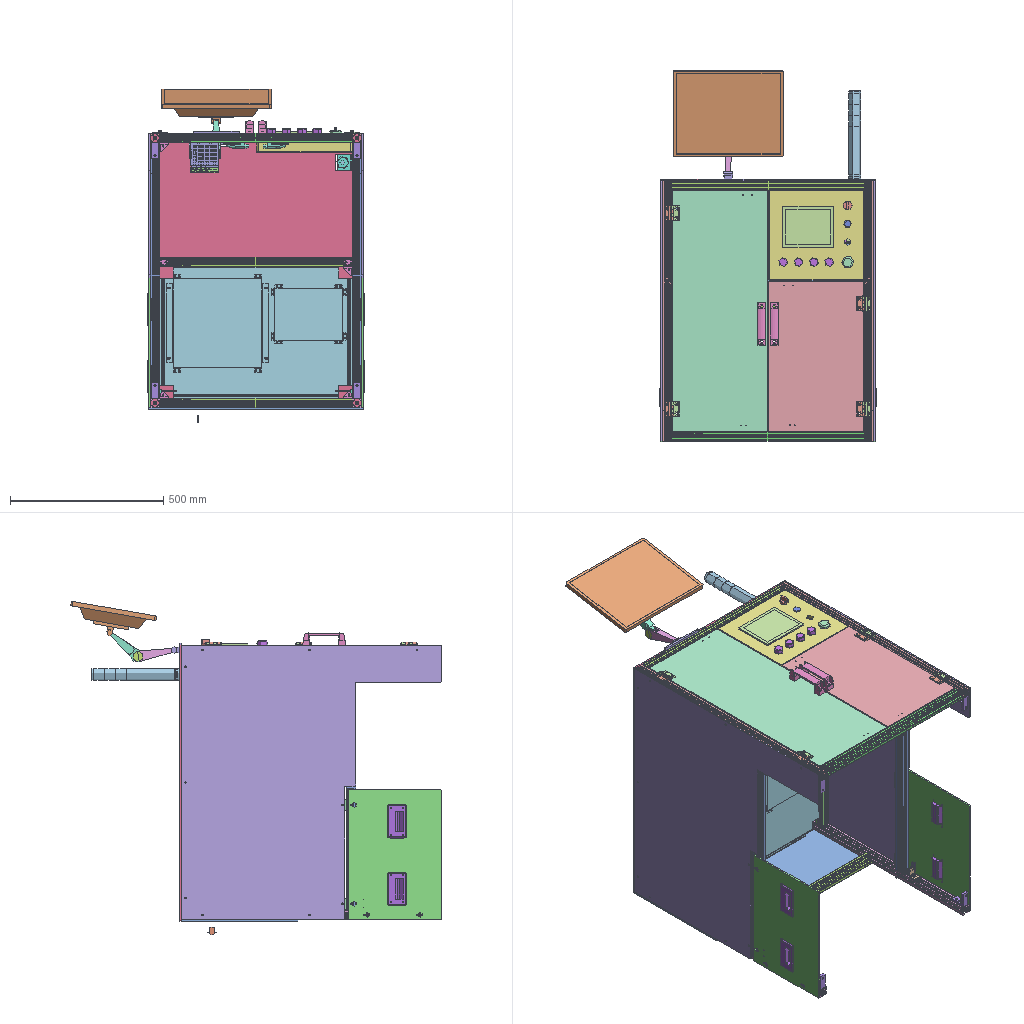Assembly | STEP file | 62 different items | 138 placed | box 710 x 1211 x 1090 mm
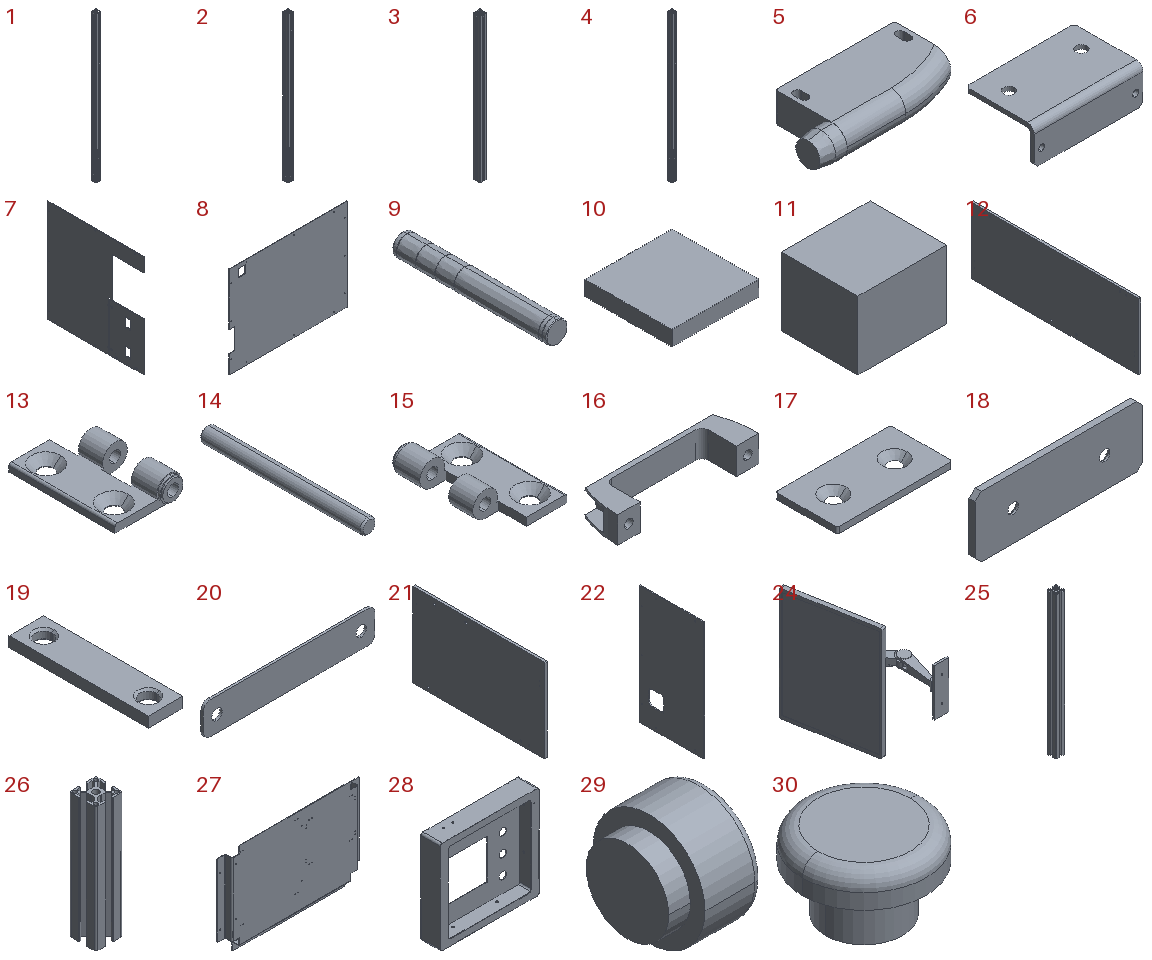Parts list (item | name | quantity | parent item | size | volume):
1 | 227H056139_Default | x2 | in 20 | 30 x 30 x 850 mm | 322963 mm3
2 | SQ-8-3030W-835_Default | x4 | in 20 | 30 x 30 x 835 mm | 317751 mm3
3 | SQ-8-3030W-630_Default | x4 | in 20 | 30 x 30 x 630 mm | 238380 mm3
4 | SQ-8-3030W-850_Default | x2 | in 20 | 30 x 30 x 850 mm | 323559 mm3
5 | AZC11013Y_Default | x2 | in 20 | 72.7 x 40.3 x 15 mm | 31534 mm3
6 | 227H056122 Sensor BKT_Default | x1 | in 20 | 60 x 38 x 20 mm | 7342 mm3
7 | 227H056116 Side Cover _Default | x2 | in 20 | 5 x 849 x 893 mm | 3234817 mm3
8 | 227H056117 Top Cover_Default | x1 | in 20 | 900 x 5 x 700 mm | 3097744 mm3
9 | SceondRR_Default | x1 | in 20 | 40 x 289 x 40 mm | 362543 mm3
10 | SceondUPS_Default | x1 | in 20 | 290 x 290 x 50 mm | 4205000 mm3
11 | SceondREWTRT_Default | x1 | in 20 | 220 x 190 x 170 mm | 7106000 mm3
12 | 227H056118 DOOR L_Default | x1 | in DOOR L_Default | 10 x 786 x 311 mm | 2441721 mm3
13 | SecondRearHHPMGS6p1_Default | x4 | in HHPMGS6_Default | 29.5 x 48.7 x 11 mm | 4355 mm3
14 | SecondRearHHPMGS6pin_Default | x4 | in HHPMGS6_Default | 5 x 54 x 5 mm | 1057 mm3
15 | SecondRearHHPMGS6p2_Default | x4 | in HHPMGS6_Default | 29.5 x 48.7 x 11 mm | 4355 mm3
16 | SecondRearUPCN26-B-41_b_Default | x2 | in DOOR L_Default, DOOR R_Default | 139 x 41 x 26 mm | 37829 mm3
17 | SceondC-100-B-2Receiving Plate_Default | x2 | in DOOR L_Default, DOOR R_Default | 30 x 16 x 1.6 mm | 705.168 mm3
18 | Part1.SLDPRTrtt_Default | x2 | in DOOR L_Default, DOOR R_Default | 55 x 2 x 20 mm | 2119 mm3
19 | hhpnt6_2_2_03 | x4 | in DOOR L_Default, DOOR R_Default | 10 x 40 x 3 mm | 1076 mm3
20 | upcnat117_2_03 | x2 | in DOOR L_Default, DOOR R_Default | 139 x 2 x 26 mm | 6946 mm3
21 | 227H056119 DOOR R_Default | x1 | in DOOR R_Default | 10 x 491 x 311 mm | 1524271 mm3
22 | 227H056124 Rear Cover SLDPRT_Default | x1 | in 20 | 5 x 380 x 700 mm | 1290724 mm3
23 | 0-ARK-3500_Default | x1 | in 20 | - | -
24 | TV | x1 | in 20 | 197.95 x 360.761 x 359.449 mm | 3578288 mm3
25 | SQ-8-3030W-460_Default | x2 | in 20 | 30 x 30 x 460 mm | 172560 mm3
26 | SQ-8-3030W-160_Default | x2 | in 20 | 30 x 30 x 140 mm | 48663 mm3
27 | 227H056121 BKT_Default | x1 | in 20 | 685.4 x 35.3 x 457.7 mm | 768690 mm3
28 | 227H056120A Front Panel | x1 | in Front Panel | 313 x 61.6 x 295 mm | 263384 mm3
29 | 7-4-Part3-619-724 | x4 | in Front Panel | 21.06 x 29.813 x 29.813 mm | 12789 mm3
30 | 7-4-Emergency Stop Button1-619-724_Default | x1 | in Front Panel | 40 x 40 x 25 mm | 19293 mm3
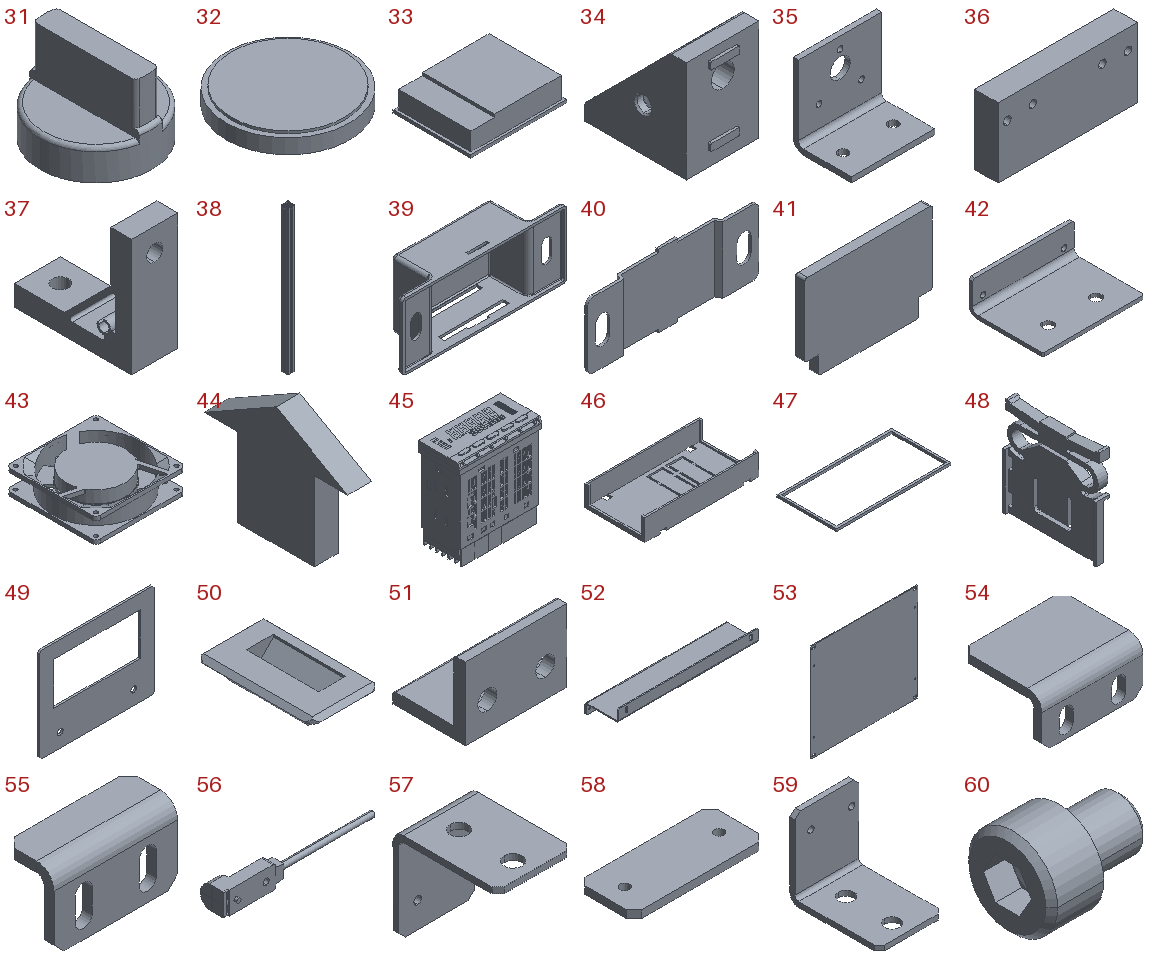31 | 7-4-Switch1-619-724_Default | x1 | in Front Panel | 29 x 29 x 21 mm | 7372 mm3
32 | 7-4-Button1-619-724_Default | x1 | in Front Panel | 25 x 25 x 3.5 mm | 1680 mm3
33 | Display-724_Default | x1 | in Front Panel | 165 x 134 x 41 mm | 776017 mm3
34 | - | x19 | in 20 | 20 x 28.7 x 28.7 mm | 5707 mm3
35 | 203H124123 Signal Tower BKT_Default | x1 | in 20 | 50 x 35 x 48 mm | 11822 mm3
36 | 227H056123 Block_Default | x1 | in 20 | 60 x 10 x 30 mm | 17658 mm3
37 | hblts6_2_03 | x4 | in 20 | 20 x 51 x 51 mm | 16227 mm3
38 | SQ-8-3030W-630 Bottom_Default | x1 | in 20 | 30 x 30 x 630 mm | 237831 mm3
39 | SceondC-100-B-2Case_Default | x2 | in SceondC-100-B-2, C-100-B-2 | 56.5 x 15.3 x 23 mm | 2154 mm3
40 | SceondC-100-B-2Base Plate_Default | x2 | in SceondC-100-B-2, C-100-B-2 | 54.5 x 2.5 x 23 mm | 897.584 mm3
41 | SceondC-100-BYoke_Default | x2 | in SceondC-100-BYoke_Male_Default | 28 x 2 x 20 mm | 1071 mm3
42 | 227H056396 BKT_Default | x2 | in 20 | 56.5 x 41.063 x 18 mm | 6109 mm3
43 | 1_2_1-- | x1 | in E0141_Default | 92 x 92 x 25 mm | 97841 mm3
44 | 2_2_1-- | x1 | in E0141_Default | 5 x 30 x 25 mm | 1957 mm3
45 | K3HB_V_BASE | x1 | in K3HB_V | 96 x 48 x 108.3 mm | 416393 mm3
46 | K3HB_V_COVER. | x1 | in K3HB_V | 91 x 47.87 x 17 mm | 10803 mm3
47 | K3HB_V_PACKING | x1 | in K3HB_V | 95 x 48.8 x 2 mm | 1118 mm3
48 | K3HB_V_ADAPTER | x2 | in K3HB_V | 6.7 x 47.4 x 49.3 mm | 5859 mm3
49 | 227H0563998 BKT_Default | x1 | in K3HB_V | 122 x 2 x 100 mm | 15991 mm3
50 | uwuan109_5_n_2_14a | x4 | in 20 | 64 x 109.5 x 19.5 mm | 44747 mm3
51 | hcba6_2_14a_Default | x4 | in 20 | 35 x 25 x 25 mm | 6095 mm3
52 | 227H056377 Guide BKT_Default | x2 | in 20 | 260 x 62 x 40 mm | 50446 mm3
53 | 227H056376 BKT_Default | x1 | in 20 | 285 x 2 x 260 mm | 147758 mm3
54 | 227H056379 BKT_Default | x8 | in 20 | 25 x 20 x 12 mm | 1357 mm3
55 | 227H056378 BKT_Default | x4 | in 20 | 25 x 10 x 15 mm | 978.865 mm3
56 | gx-h12a | x2 | in 20 | 81.8 x 14.5 x 12 mm | 2908 mm3
57 | 227H056375 Sensor BKT_Default | x1 | in 20 | 25 x 35 x 31 mm | 2998 mm3
58 | 227H056374 Sensor Dog_Default | x2 | in 20 | 35 x 15 x 2 mm | 1014 mm3
59 | 227H056373 Sensor BKT_Default | x1 | in 20 | 25 x 35 x 31 mm | 2998 mm3
60 | CB5-6_Default | x1 | in CB5-6_SW5_W5_Default | 11 x 8.5 x 8.5 mm | 358.786 mm3
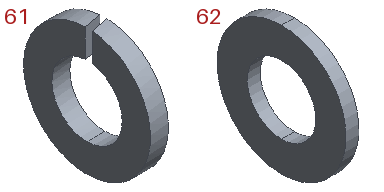61 | SW5_Default | x1 | in CB5-6_SW5_W5_Default | 1.3 x 9.2 x 9.198 mm | 58.481 mm3
62 | W5_Default | x1 | in CB5-6_SW5_W5_Default | 1 x 10 x 10 mm | 56.478 mm3
Placements (level | parent | child | x y z in mm | rotation matrix by rows):
1 | 20 | 227H056139_Default | -330.0 175.4 435.0 | -1 0 0 0 0 -1 0 -1 0
1 | 20 | SQ-8-3030W-835_Default | -330.0 835.0 244.6 | 1 0 0 0 1 0 0 0 1
1 | 20 | SQ-8-3030W-835_Default | 330.0 835.0 244.6 | 1 0 0 0 1 0 0 0 1
1 | 20 | SQ-8-3030W-630_Default | -139.6 835.0 -430.0 | 0 0 -1 -1 0 0 0 1 -0
1 | 20 | SQ-8-3030W-630_Default | -139.6 835.0 435.0 | 0 0 -1 -1 0 0 0 1 -0
1 | 20 | 227H056139_Default | 330.0 175.4 435.0 | 1 0 0 0 0 -1 0 1 0
1 | 20 | SQ-8-3030W-850_Default | -330.0 674.6 -430.0 | 0 1 0 0 0 1 1 0 0
1 | 20 | SQ-8-3030W-850_Default | 330.0 674.6 -430.0 | 0 1 0 0 0 1 1 0 0
1 | 20 | AZC11013Y_Default | -37 796.0 401.389 | -1 0 0 0 0 1 0 1 -0
1 | 20 | 227H056122 Sensor BKT_Default | -66.999 811.0 414.7 | -1 0 0 0 1 0 0 0 -1
1 | 20 | AZC11013Y_Default | 37 515.0 400.411 | 1 0 0 0 0 -1 0 1 -0
1 | 20 | 227H056116 Side Cover _Default | -350.0 424.5 2.5 | 1 0 0 0 1 0 0 0 1
1 | 20 | 227H056116 Side Cover _Default | 345.0 424.5 2.5 | 1 0 0 0 1 0 0 0 1
1 | 20 | 227H056117 Top Cover_Default | -0.0 850.0 -0.0 | 0 0 1 0 1 0 -1 0 0
1 | 20 | SceondRR_Default | 283.5 855.0 355.0 | -0.9502 0 0.3116 0 1 0 -0.3116 0 -0.9502
1 | 20 | SceondUPS_Default | -270.7 699.3 -25.0 | 1 0 0 0 0 1 0 -1 0
1 | 20 | SceondREWTRT_Default | 172.0 649.3 -140.0 | -1 0 0 0 1 0 0 0 -1
1 | 20 | DOOR L_Default | -157.5 425.0 440.0 | 0 0 -1 0 1 0 1 0 -0
2 | DOOR L_Default | 227H056118 DOOR L_Default | -0.0 -0.0 -0.0 | 1 0 0 0 1 0 0 0 1
2 | DOOR L_Default | HHPMGS6_Default | 15.5 319.5 156.5 | 0 0 1 0 1 0 -1 0 -0
3 | HHPMGS6_Default | SecondRearHHPMGS6p1_Default | 0.0 0.0 -0.0 | 1 0 0 0 1 0 0 0 1
3 | HHPMGS6_Default | SecondRearHHPMGS6pin_Default | 0.0 0.0 -0.0 | 1 0 0 0 1 0 0 0 1
3 | HHPMGS6_Default | SecondRearHHPMGS6p2_Default | 0.0 0.0 -0.0 | 1 0 0 0 1 0 0 0 1
2 | DOOR L_Default | SecondRearUPCN26-B-41_b_Default | 10.0 16.3 -137.5 | 0 1 0 -1 0 0 0 0 1
2 | DOOR L_Default | HHPMGS6_Default | 15.5 -319.5 156.5 | 0 0 1 0 1 0 -1 0 -0
3 | HHPMGS6_Default | SecondRearHHPMGS6p1_Default | 0.0 0.0 -0.0 | 1 0 0 0 1 0 0 0 1
3 | HHPMGS6_Default | SecondRearHHPMGS6pin_Default | 0.0 0.0 -0.0 | 1 0 0 0 1 0 0 0 1
3 | HHPMGS6_Default | SecondRearHHPMGS6p2_Default | 0.0 0.0 -0.0 | 1 0 0 0 1 0 0 0 1
2 | DOOR L_Default | SceondC-100-B-2Receiving Plate_Default | -1.6 -381.7 -78.2 | 0 0 -1 0 1 0 1 0 -0
2 | DOOR L_Default | Part1.SLDPRTrtt_Default | -0.0 378.0 -90.5 | 0 -1 0 0 0 -1 1 0 0
2 | DOOR L_Default | hhpnt6_2_2_03 | 0.0 319.5 140.5 | 0 0 -1 0 1 0 1 0 0
2 | DOOR L_Default | hhpnt6_2_2_03 | -0.0 -319.5 140.5 | 0 0 -1 0 1 0 1 0 0
2 | DOOR L_Default | upcnat117_2_03 | 0.0 -42.2 -137.5 | 0 -1 0 1 0 0 0 0 1
1 | 20 | DOOR R_Default | 157.5 277.5 440.0 | 0 0 -1 0 1 0 1 0 -0
2 | DOOR R_Default | 227H056119 DOOR R_Default | -0.0 -0.0 -0.0 | 1 0 0 0 1 0 0 0 1
2 | DOOR R_Default | SecondRearUPCN26-B-41_b_Default | 10.0 46.8 137.5 | 0 1 0 1 0 0 0 0 -1
2 | DOOR R_Default | SceondC-100-B-2Receiving Plate_Default | -1.6 -233.7 78.2 | 0 0 -1 0 1 0 1 0 -0
2 | DOOR R_Default | HHPMGS6_Default | 15.5 -172.0 -156.5 | 0 0 1 0 1 0 -1 0 -0
3 | HHPMGS6_Default | SecondRearHHPMGS6p1_Default | 0.0 0.0 -0.0 | 1 0 0 0 1 0 0 0 1
3 | HHPMGS6_Default | SecondRearHHPMGS6pin_Default | 0.0 0.0 -0.0 | 1 0 0 0 1 0 0 0 1
3 | HHPMGS6_Default | SecondRearHHPMGS6p2_Default | 0.0 0.0 -0.0 | 1 0 0 0 1 0 0 0 1
2 | DOOR R_Default | HHPMGS6_Default | 15.5 172.0 -156.5 | 0 0 1 0 1 0 -1 0 -0
3 | HHPMGS6_Default | SecondRearHHPMGS6p1_Default | 0.0 0.0 -0.0 | 1 0 0 0 1 0 0 0 1
3 | HHPMGS6_Default | SecondRearHHPMGS6pin_Default | 0.0 0.0 -0.0 | 1 0 0 0 1 0 0 0 1
3 | HHPMGS6_Default | SecondRearHHPMGS6p2_Default | 0.0 0.0 -0.0 | 1 0 0 0 1 0 0 0 1
2 | DOOR R_Default | Part1.SLDPRTrtt_Default | 0.0 230.5 90.5 | 0 -1 0 0 0 -1 1 0 -0
2 | DOOR R_Default | hhpnt6_2_2_03 | -0.0 172.0 -140.5 | 0 0 -1 0 -1 0 -1 0 0
2 | DOOR R_Default | hhpnt6_2_2_03 | 0.0 -172.0 -140.5 | 0 0 -1 0 -1 0 -1 0 0
2 | DOOR R_Default | upcnat117_2_03 | -2.0 105.3 137.5 | 0 1 0 -1 0 0 0 0 1
1 | 20 | 227H056124 Rear Cover SLDPRT_Default | -0.0 659.0 -445.0 | 0 0 1 0 1 0 -1 0 0
1 | 20 | 0-ARK-3500_Default | -125 776.3 -57.0 | 1 0 0 0 1 0 0 0 1
1 | 20 | TV | -130.0 991.0 414.162 | 0 0 1 0 1 0 -1 0 0
1 | 20 | SQ-8-3030W-630_Default | -139.6 835.0 30.0 | 0 0 -1 -1 0 0 0 1 -0
1 | 20 | SQ-8-3030W-460_Default | -330.0 665.0 -130.4 | 1 0 0 0 1 0 0 0 1
1 | 20 | SQ-8-3030W-460_Default | 330.0 665.0 -130.4 | 1 0 0 0 1 0 0 0 1
1 | 20 | SQ-8-3030W-160_Default | -330.0 855.4 30.0 | 1 0 0 0 0 -1 0 1 -0
1 | 20 | SQ-8-3030W-160_Default | 330.0 855.4 30.0 | 1 0 0 0 0 -1 0 1 -0
1 | 20 | 227H056121 BKT_Default | -0.0 649.3 -197.3 | 1 0 0 0 1 0 0 0 1
1 | 20 | SQ-8-3030W-630_Default | -139.6 431.238 -430.0 | 0 0 -1 -1 0 0 0 1 -0
1 | 20 | Front Panel | 353.404 -309.683 99.086 | 0.9984 -0.05571 0.009823 0.05657 0.9832 -0.1734 0 0.1736 0.9848
2 | Front Panel | 227H056120A Front Panel | -158.206 1026.246 175.373 | 0.9984 0 -0.05657 -0.05571 0.1736 -0.9832 0.009823 0.9848 0.1734
2 | Front Panel | 7-4-Part3-619-724 | -254.243 966.693 180.016 | 0 -0.1736 -0.9848 0.1736 0.9698 -0.171 0.9848 -0.171 0.03015
2 | Front Panel | 7-4-Part3-619-724 | -204.323 963.907 180.507 | 0 -0.1736 -0.9848 0.1736 0.9698 -0.171 0.9848 -0.171 0.03015
2 | Front Panel | 7-4-Part3-619-724 | -154.404 961.122 180.998 | 0 -0.1736 -0.9848 0.1736 0.9698 -0.171 0.9848 -0.171 0.03015
2 | Front Panel | 7-4-Part3-619-724 | -104.484 958.336 181.489 | 0 -0.1736 -0.9848 0.1736 0.9698 -0.171 0.9848 -0.171 0.03015
2 | Front Panel | 7-4-Emergency Stop Button1-619-724_Default | -42.67 947.063 199.489 | 1 0 0 0 0.9848 0.1736 0 -0.1736 0.9848
2 | Front Panel | 7-4-Switch1-619-724_Default | -32.204 1130.871 178.249 | 1 0 0 0 0.9848 0.1736 0 -0.1736 0.9848
2 | Front Panel | 7-4-Button1-619-724_Default | -35.598 1068.752 170.924 | 1 0 0 0 0.9848 0.1736 0 -0.1736 0.9848
2 | Front Panel | Display-724_Default | -177.335 1078.541 171.229 | 0.9984 -0.05657 0 -0.05571 -0.9832 -0.1736 0.009823 0.1734 -0.9848
1 | 20 | subassembly 2 | -330.0 820.0 -415.0 | 1 0 0 0 0 -1 0 1 0
1 | 20 | subassembly 2 | -330.0 680.0 -415.0 | -1 0 0 0 0 1 0 1 -0
1 | 20 | subassembly 2 | -330.0 680.0 15.0 | -1 0 0 0 1 0 0 0 -1
1 | 20 | subassembly 2 | -330.0 820.0 15.0 | -1 0 0 0 0 -1 0 -1 -0
1 | 20 | subassembly 2 | 330.0 820.0 420.0 | -1 0 0 0 0 -1 0 -1 0
1 | 20 | subassembly 2 | 330.0 820.0 45.0 | -1 0 0 0 -1 0 0 0 1
1 | 20 | subassembly 2 | 315.0 680.0 30.0 | 0 0 -1 0 1 0 1 0 0
1 | 20 | subassembly 2 | -315.0 680.0 30.0 | 0 0 1 0 1 0 -1 0 0
1 | 20 | subassembly 2 | 315.0 665.0 15.0 | 0 0 -1 1 0 0 0 -1 -0
1 | 20 | subassembly 2 | 315.0 820.0 30.0 | 0 -1 0 0 0 -1 1 0 -0
1 | 20 | subassembly 2 | -315.0 820.0 30.0 | 0 1 0 0 0 -1 -1 0 -0
1 | 20 | subassembly 2 | -330.0 820.0 45.0 | -1 0 0 0 -1 0 0 0 1
1 | 20 | subassembly 2 | -330.0 820.0 420.0 | -1 0 0 0 0 -1 0 -1 0
1 | 20 | subassembly 2 | 315.0 820.0 -430.0 | 0 -1 0 0 0 -1 1 0 -0
1 | 20 | subassembly 2 | -315.0 820.0 -430.0 | 0 1 0 0 0 -1 -1 0 -0
1 | 20 | subassembly 2 | -315.0 835.0 420.0 | 0 1 0 1 0 0 0 0 -1
1 | 20 | subassembly 2 | 315.0 835.0 420.0 | 0 0 -1 1 0 0 0 -1 -0
1 | 20 | subassembly 2 | 315.0 835.0 -415.0 | 0 0 -1 -1 0 0 0 1 -0
1 | 20 | subassembly 2 | -315.0 835.0 -415.0 | 0 1 0 -1 0 0 0 0 1
1 | 20 | 203H124123 Signal Tower BKT_Default | 315.0 820.0 355.0 | 0 0 -1 0 1 0 1 0 -0
1 | 20 | 227H056123 Block_Default | 67.0 515.0 421.3 | 1 0 0 0 1 0 0 0 1
1 | 20 | hblts6_2_03 | -330.0 0.0 420.0 | 1 0 0 0 0 1 0 -1 -0
1 | 20 | hblts6_2_03 | 330.0 0.0 420.0 | 1 0 0 0 0 1 0 -1 -0
1 | 20 | hblts6_2_03 | 330.0 0.0 -415.0 | -1 0 0 0 0 1 0 1 -0
1 | 20 | hblts6_2_03 | -330.0 0.0 -415.0 | -1 0 0 0 0 1 0 1 -0
1 | 20 | SQ-8-3030W-630 Bottom_Default | -139.6 15.0 435.0 | 0 0 -1 1 0 0 0 -1 -0
1 | 20 | SceondC-100-B-2 | -79.3 44.0 425.7 | -1 0 0 0 1 0 0 0 -1
2 | SceondC-100-B-2 | SceondC-100-B-2Case_Default | -0.0 -0.0 -0.0 | 1 0 0 0 1 0 0 0 1
2 | SceondC-100-B-2 | SceondC-100-B-2Base Plate_Default | -0.0 0.3 -0.0 | 1 0 0 0 1 0 0 0 1
2 | SceondC-100-B-2 | SceondC-100-BYoke_Male_Default | -0.0 2.8 -0.0 | 1 0 0 0 1 0 0 0 1
3 | SceondC-100-BYoke_Male_Default | SceondC-100-BYoke_Default | -0.0 9.0 -0.0 | 1 0 0 0 1 0 0 0 1
1 | 20 | C-100-B-2 | 79.3 44.0 425.7 | -1 0 0 0 1 0 0 0 -1
2 | C-100-B-2 | SceondC-100-B-2Case_Default | -0.0 -0.0 -0.0 | 1 0 0 0 1 0 0 0 1
2 | C-100-B-2 | SceondC-100-B-2Base Plate_Default | 0.0 0.3 -0.0 | 1 0 0 0 1 0 0 0 1
2 | C-100-B-2 | SceondC-100-BYoke_Male_Default | 0.0 2.8 -0.0 | 1 0 0 0 1 0 0 0 1
3 | SceondC-100-BYoke_Male_Default | SceondC-100-BYoke_Default | -0.0 9.0 -0.0 | 1 0 0 0 1 0 0 0 1
1 | 20 | 227H056396 BKT_Default | 67.55 44.0 418.0 | 1 0 0 0 1 0 0 0 1
1 | 20 | 227H056396 BKT_Default | -91.05 44.0 418.0 | 1 0 0 0 1 0 0 0 1
1 | 20 | E0141_Default | -190.0 749.0 -445.0 | -1 0 0 0 1 0 0 0 -1
2 | E0141_Default | 1_2_1-- | -0.0 -0.0 -0.0 | 1 0 0 0 1 0 0 0 1
2 | E0141_Default | 2_2_1-- | -0.0 -0.0 -0.0 | 1 0 0 0 1 0 0 0 1
1 | 20 | K3HB_V | -167.0 787.6 419.996 | 1 0 0 0 1 0 0 0 1
2 | K3HB_V | K3HB_V_BASE | -0.0 -0.0 -0.0 | 1 0 0 0 1 0 0 0 1
2 | K3HB_V | K3HB_V_COVER. | 0.0188 -0.0 -81.0 | -1 0 0 0 -1 0 0 0 1
2 | K3HB_V | K3HB_V_PACKING | -0.0 -0.0 0.0038 | 1 0 0 0 1 0 0 0 1
2 | K3HB_V | K3HB_V_ADAPTER | 45.6 -0.0 -2.517 | 1 0 0 0 1 0 0 0 1
2 | K3HB_V | K3HB_V_ADAPTER | -45.6 0.0 -3.183 | -1 0 0 0 -1 0 0 0 1
2 | K3HB_V | 227H0563998 BKT_Default | 0.4 12.4 2.004 | 1 0 0 0 0 -1 0 1 -0
1 | 20 | uwuan109_5_n_2_14a | 350.0 145.0 -124.75 | 0 0 1 -1 0 0 0 -1 0
1 | 20 | uwuan109_5_n_2_14a | 350.0 145.0 -344.75 | 0 0 1 -1 0 0 0 -1 0
1 | 20 | SQ-8-3030W-835_Default | 330.0 295.0 244.6 | 1 0 0 0 1 0 0 0 1
1 | 20 | hcba6_2_14a_Default | 340.0 310.0 -71.314 | 0 0 -1 0 1 0 1 0 0
1 | 20 | 227H056377 Guide BKT_Default | -272.7 651.3 -299.5 | 0 0 -1 0 1 0 1 0 -0
1 | 20 | 227H056377 Guide BKT_Default | 21.3 651.3 -39.5 | 0 0 1 0 1 0 -1 0 0
1 | 20 | 227H056376 BKT_Default | -125.7 713.3 -169.5 | 1 0 0 0 1 0 0 0 1
1 | 20 | 227H056379 BKT_Default | 282.0 649.3 -80.0 | 0 0 -1 0 1 0 1 0 -0
1 | 20 | 227H056379 BKT_Default | 62.0 649.3 -55.0 | 0 0 1 0 1 0 -1 0 -0
1 | 20 | 227H056379 BKT_Default | 62.0 649.3 -200.0 | 0 0 1 0 1 0 -1 0 -0
1 | 20 | 227H056379 BKT_Default | 282.0 649.3 -225.0 | 0 0 -1 0 1 0 1 0 -0
1 | 20 | 227H056379 BKT_Default | 87.0 649.3 -55.0 | -1 0 0 0 1 0 0 0 -1
1 | 20 | 227H056379 BKT_Default | 282.0 649.3 -55.0 | -1 0 0 0 1 0 0 0 -1
1 | 20 | 227H056379 BKT_Default | 257.0 649.3 -225.0 | 1 0 0 0 1 0 0 0 1
1 | 20 | 227H056379 BKT_Default | 62.0 649.3 -225.0 | 1 0 0 0 1 0 0 0 1
1 | 20 | 227H056378 BKT_Default | -245.7 649.3 -25.0 | -1 0 0 0 1 0 0 0 -1
1 | 20 | 227H056378 BKT_Default | -5.7 649.3 -315.0 | 1 0 0 0 1 0 0 0 1
1 | 20 | 227H056378 BKT_Default | -270.7 649.3 -315.0 | 1 0 0 0 1 0 0 0 1
1 | 20 | 227H056378 BKT_Default | 19.3 649.3 -25.0 | -1 0 0 0 1 0 0 0 -1
1 | 20 | gx-h12a | -318.8 249.108 -392.5 | 1 0 0 0 1 0 0 0 1
1 | 20 | 227H056375 Sensor BKT_Default | 328.5 248.0 -398.5 | -1 0 0 0 1 0 0 0 -1
1 | 20 | 227H056374 Sensor Dog_Default | 345.0 247.0 -410.0 | 0 0 1 0 1 0 -1 0 0
1 | 20 | SQ-8-3030W-835_Default | -330.0 295.0 244.6 | 1 0 0 0 1 0 0 0 1
1 | 20 | 227H056374 Sensor Dog_Default | -345.0 262.0 -410.0 | 0 0 -1 0 -1 0 -1 0 -0
1 | 20 | 227H056373 Sensor BKT_Default | -328.5 249.108 -398.5 | 1 0 0 0 1 0 0 0 1
1 | 20 | gx-h12a | 318.8 248.0 -392.5 | -1 0 0 0 1 0 0 0 -1
1 | 20 | CB5-6_SW5_W5_Default | 330.372 235.477 -411.922 | 0 0.2122 0.9772 0 0.9772 -0.2122 -1 0 -0
2 | CB5-6_SW5_W5_Default | CB5-6_Default | -1.222 1.409 -0.6868 | 1 0 0 0 1 0 0 0 1
2 | CB5-6_SW5_W5_Default | SW5_Default | -0.572 1.409 -0.6868 | 1 0 0 0 1 0 0 0 1
2 | CB5-6_SW5_W5_Default | W5_Default | 0.578 1.409 -0.6868 | 1 0 0 0 0.9999 0.01201 0 -0.01201 0.9999
1 | 20 | hcba6_2_14a_Default | 340.0 310.0 -393.437 | 0 0 -1 0 1 0 1 0 0
1 | 20 | hcba6_2_14a_Default | -345.0 310.0 -393.311 | 0 0 1 0 1 0 -1 0 -0
1 | 20 | hcba6_2_14a_Default | -345.0 310.0 -71.875 | 0 0 1 0 1 0 -1 0 -0
1 | 20 | uwuan109_5_n_2_14a | -350.0 145.0 -344.75 | 0 0 -1 -1 0 0 0 1 0
1 | 20 | uwuan109_5_n_2_14a | -350.0 145.0 -124.75 | 0 0 -1 -1 0 0 0 1 0